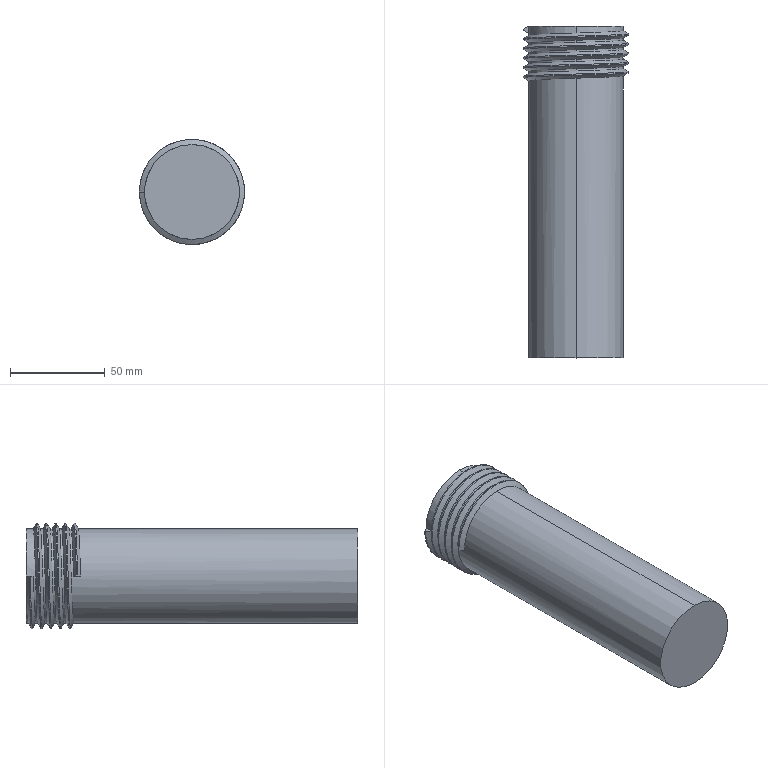Part | SolidWorks | features Extrusion 1, SweepThread 1 | 1 solid | 19 faces | box 55.413 x 175 x 55.413 mm | volume 348440 mm3 | cylinder 12 | plane 4 | spline 3 | commonest cylinder face diameters 50 x12